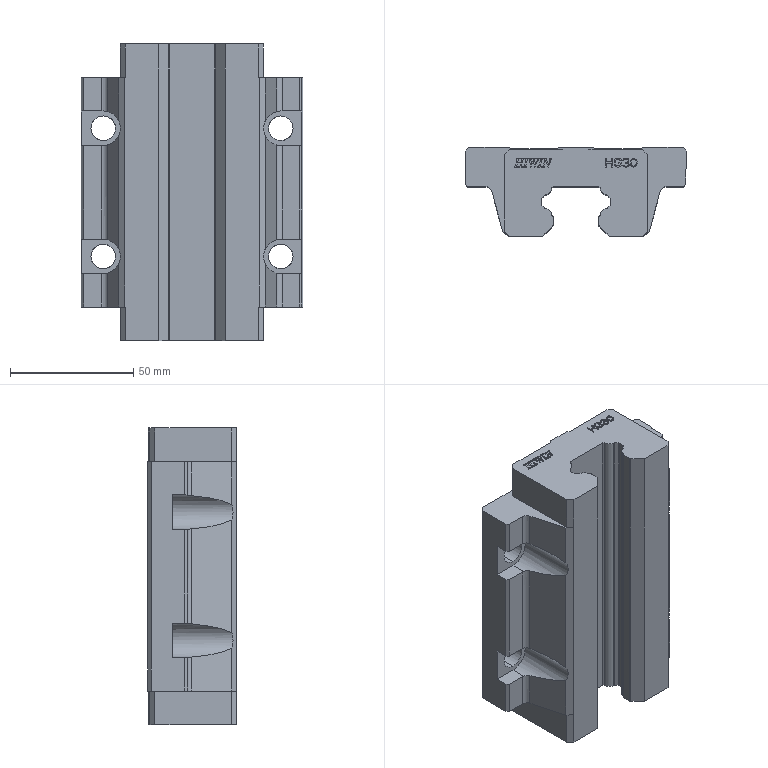Part | STEP file | slider HGW30HC | 1 solid | 426 faces | box 90 x 36 x 120.7 mm | volume 241575 mm3 | plane 328 | spline 60 | cylinder 38 | commonest cylinder face diameters 1.2 x12 10 x8 5 x6 1.6 x4 5.66 x4 14 x4